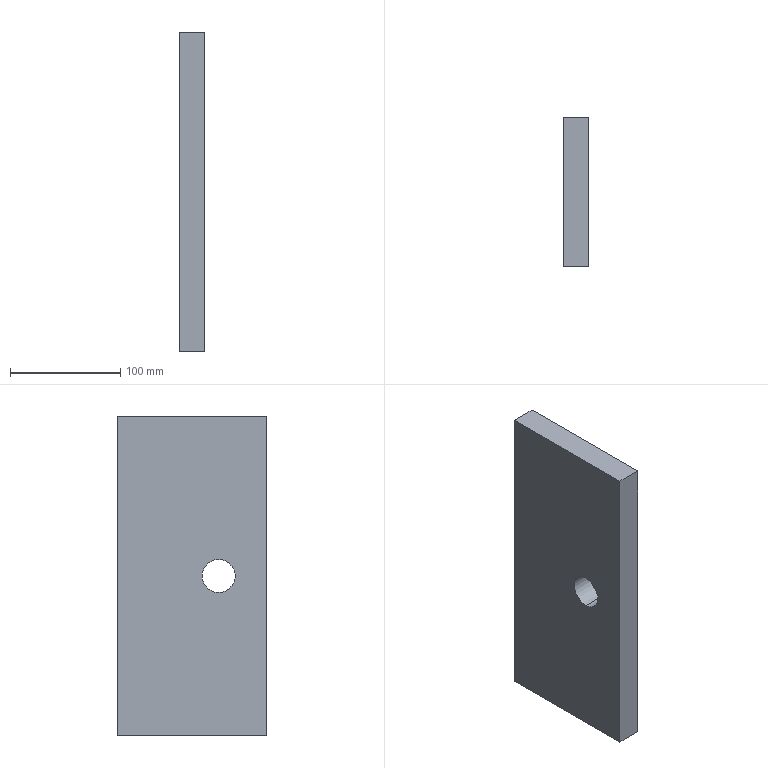Part | SolidWorks | features BaseBody 1 | 1 solid | 13 faces | box 22.77 x 135.5 x 290 mm | volume 870909 mm3 | plane 8 | cylinder 5 | commonest cylinder face diameters 73.25 x3 30 x2
STEP:
#1=CARTESIAN_POINT('',(-12.5,-26.5,-15.));
#2=VERTEX_POINT('',#1);
#3=CARTESIAN_POINT('',(-12.5,-26.5,15.));
#4=VERTEX_POINT('',#3);
#5=CARTESIAN_POINT('',(-12.5,-26.5,0.));
#6=DIRECTION('',(-1.,0.,0.));
#7=DIRECTION('',(0.,0.,-1.));
#8=AXIS2_PLACEMENT_3D('',#5,#6,#7);
#9=CIRCLE('',#8,15.);
#10=EDGE_CURVE('',#2,#4,#9,.T.);
#11=ORIENTED_EDGE('',*,*,#10,.T.);
#12=CARTESIAN_POINT('',(8.04,-26.5,15.));
#13=VERTEX_POINT('',#12);
#14=CARTESIAN_POINT('',(-12.501,-26.5,15.));
#15=DIRECTION('',(1.,0.,0.));
#16=VECTOR('',#15,1000.);
#17=LINE('',#14,#16);
#18=EDGE_CURVE('',#4,#13,#17,.T.);
#19=ORIENTED_EDGE('',*,*,#18,.T.);
#20=CARTESIAN_POINT('',(8.04,-26.5,-15.));
#21=VERTEX_POINT('',#20);
#22=CARTESIAN_POINT('',(8.04,-26.5,0.));
#23=DIRECTION('',(-1.,0.,0.));
#24=DIRECTION('',(0.,0.,-1.));
#25=AXIS2_PLACEMENT_3D('',#22,#23,#24);
#26=CIRCLE('',#25,15.);
#27=EDGE_CURVE('',#21,#13,#26,.T.);
#28=ORIENTED_EDGE('',*,*,#27,.F.);
#29=CARTESIAN_POINT('',(-12.501,-26.5,-15.));
#30=DIRECTION('',(1.,0.,0.));
#31=VECTOR('',#30,1000.);
#32=LINE('',#29,#31);
#33=EDGE_CURVE('',#2,#21,#32,.T.);
#34=ORIENTED_EDGE('',*,*,#33,.F.);
#35=EDGE_LOOP('',(#11,#19,#28,#34));
#36=FACE_OUTER_BOUND('',#35,.T.);
#37=CARTESIAN_POINT('',(-12.501,-26.5,0.));
#38=DIRECTION('',(1.,0.,0.));
#39=DIRECTION('',(0.,0.,-1.));
#40=AXIS2_PLACEMENT_3D('',#37,#38,#39);
#41=CYLINDRICAL_SURFACE('',#40,15.);
#42=ADVANCED_FACE('',(#36),#41,.F.);
#43=CARTESIAN_POINT('',(8.04,-26.5,36.625));
#44=VERTEX_POINT('',#43);
#45=CARTESIAN_POINT('',(8.04,-61.,12.294));
#46=VERTEX_POINT('',#45);
#47=CARTESIAN_POINT('',(8.04,-26.5,0.));
#48=DIRECTION('',(1.,0.,0.));
#49=DIRECTION('',(0.,0.,-1.));
#50=AXIS2_PLACEMENT_3D('',#47,#48,#49);
#51=CIRCLE('',#50,36.625);
#52=EDGE_CURVE('',#44,#46,#51,.T.);
#53=ORIENTED_EDGE('',*,*,#52,.F.);
#54=CARTESIAN_POINT('',(10.27,-26.5,36.625));
#55=VERTEX_POINT('',#54);
#56=CARTESIAN_POINT('',(8.04,-26.5,36.625));
#57=DIRECTION('',(1.,0.,0.));
#58=VECTOR('',#57,1000.);
#59=LINE('',#56,#58);
#60=EDGE_CURVE('',#44,#55,#59,.T.);
#61=ORIENTED_EDGE('',*,*,#60,.T.);
#62=CARTESIAN_POINT('',(10.27,-61.,12.294));
#63=VERTEX_POINT('',#62);
#64=CARTESIAN_POINT('',(10.27,-26.5,0.));
#65=DIRECTION('',(1.,0.,0.));
#66=DIRECTION('',(0.,0.,-1.));
#67=AXIS2_PLACEMENT_3D('',#64,#65,#66);
#68=CIRCLE('',#67,36.625);
#69=EDGE_CURVE('',#55,#63,#68,.T.);
#70=ORIENTED_EDGE('',*,*,#69,.T.);
#71=CARTESIAN_POINT('',(8.04,-61.,12.294));
#72=DIRECTION('',(1.,0.,0.));
#73=VECTOR('',#72,1000.);
#74=LINE('',#71,#73);
#75=EDGE_CURVE('',#46,#63,#74,.T.);
#76=ORIENTED_EDGE('',*,*,#75,.F.);
#77=EDGE_LOOP('',(#53,#61,#70,#76));
#78=FACE_OUTER_BOUND('',#77,.T.);
#79=CARTESIAN_POINT('',(8.04,-26.5,0.));
#80=DIRECTION('',(1.,0.,0.));
#81=DIRECTION('',(0.,0.,-1.));
#82=AXIS2_PLACEMENT_3D('',#79,#80,#81);
#83=CYLINDRICAL_SURFACE('',#82,36.625);
#84=ADVANCED_FACE('',(#78),#83,.F.);
#85=ORIENTED_EDGE('',*,*,#60,.F.);
#86=CARTESIAN_POINT('',(8.04,-26.5,-36.625));
#87=VERTEX_POINT('',#86);
#88=CARTESIAN_POINT('',(8.04,-26.5,0.));
#89=DIRECTION('',(1.,0.,0.));
#90=DIRECTION('',(0.,0.,-1.));
#91=AXIS2_PLACEMENT_3D('',#88,#89,#90);
#92=CIRCLE('',#91,36.625);
#93=EDGE_CURVE('',#87,#44,#92,.T.);
#94=ORIENTED_EDGE('',*,*,#93,.F.);
#95=CARTESIAN_POINT('',(10.27,-26.5,-36.625));
#96=VERTEX_POINT('',#95);
#97=CARTESIAN_POINT('',(8.04,-26.5,-36.625));
#98=DIRECTION('',(1.,0.,0.));
#99=VECTOR('',#98,1000.);
#100=LINE('',#97,#99);
#101=EDGE_CURVE('',#87,#96,#100,.T.);
#102=ORIENTED_EDGE('',*,*,#101,.T.);
#103=CARTESIAN_POINT('',(10.27,-26.5,0.));
#104=DIRECTION('',(1.,0.,0.));
#105=DIRECTION('',(0.,0.,-1.));
#106=AXIS2_PLACEMENT_3D('',#103,#104,#105);
#107=CIRCLE('',#106,36.625);
#108=EDGE_CURVE('',#96,#55,#107,.T.);
#109=ORIENTED_EDGE('',*,*,#108,.T.);
#110=EDGE_LOOP('',(#85,#94,#102,#109));
#111=FACE_OUTER_BOUND('',#110,.T.);
#112=CARTESIAN_POINT('',(8.04,-26.5,0.));
#113=DIRECTION('',(1.,0.,0.));
#114=DIRECTION('',(0.,0.,-1.));
#115=AXIS2_PLACEMENT_3D('',#112,#113,#114);
#116=CYLINDRICAL_SURFACE('',#115,36.625);
#117=ADVANCED_FACE('',(#111),#116,.F.);
#118=ORIENTED_EDGE('',*,*,#27,.T.);
#119=CARTESIAN_POINT('',(8.04,-26.5,0.));
#120=DIRECTION('',(-1.,0.,0.));
#121=DIRECTION('',(0.,0.,-1.));
#122=AXIS2_PLACEMENT_3D('',#119,#120,#121);
#123=CIRCLE('',#122,15.);
#124=EDGE_CURVE('',#13,#21,#123,.T.);
#125=ORIENTED_EDGE('',*,*,#124,.T.);
#126=EDGE_LOOP('',(#118,#125));
#127=FACE_BOUND('',#126,.T.);
#128=CARTESIAN_POINT('',(8.04,-61.,-12.294));
#129=VERTEX_POINT('',#128);
#130=CARTESIAN_POINT('',(8.04,-26.5,0.));
#131=DIRECTION('',(1.,0.,0.));
#132=DIRECTION('',(0.,0.,-1.));
#133=AXIS2_PLACEMENT_3D('',#130,#131,#132);
#134=CIRCLE('',#133,36.625);
#135=EDGE_CURVE('',#129,#87,#134,.T.);
#136=ORIENTED_EDGE('',*,*,#135,.T.);
#137=ORIENTED_EDGE('',*,*,#93,.T.);
#138=ORIENTED_EDGE('',*,*,#52,.T.);
#139=CARTESIAN_POINT('',(8.04,-61.,0.));
#140=DIRECTION('',(0.,0.,-1.));
#141=VECTOR('',#140,1000.);
#142=LINE('',#139,#141);
#143=EDGE_CURVE('',#46,#129,#142,.T.);
#144=ORIENTED_EDGE('',*,*,#143,.T.);
#145=EDGE_LOOP('',(#136,#137,#138,#144));
#146=FACE_OUTER_BOUND('',#145,.T.);
#147=CARTESIAN_POINT('',(8.04,-26.5,0.));
#148=DIRECTION('',(1.,0.,0.));
#149=DIRECTION('',(0.,0.,-1.));
#150=AXIS2_PLACEMENT_3D('',#147,#148,#149);
#151=PLANE('',#150);
#152=ADVANCED_FACE('',(#127,#146),#151,.T.);
#153=ORIENTED_EDGE('',*,*,#101,.F.);
#154=ORIENTED_EDGE('',*,*,#135,.F.);
#155=CARTESIAN_POINT('',(10.27,-61.,-12.294));
#156=VERTEX_POINT('',#155);
#157=CARTESIAN_POINT('',(8.04,-61.,-12.294));
#158=DIRECTION('',(-1.,0.,0.));
#159=VECTOR('',#158,1000.);
#160=LINE('',#157,#159);
#161=EDGE_CURVE('',#156,#129,#160,.T.);
#162=ORIENTED_EDGE('',*,*,#161,.F.);
#163=CARTESIAN_POINT('',(10.27,-26.5,0.));
#164=DIRECTION('',(1.,0.,0.));
#165=DIRECTION('',(0.,0.,-1.));
#166=AXIS2_PLACEMENT_3D('',#163,#164,#165);
#167=CIRCLE('',#166,36.625);
#168=EDGE_CURVE('',#156,#96,#167,.T.);
#169=ORIENTED_EDGE('',*,*,#168,.T.);
#170=EDGE_LOOP('',(#153,#154,#162,#169));
#171=FACE_OUTER_BOUND('',#170,.T.);
#172=CARTESIAN_POINT('',(8.04,-26.5,0.));
#173=DIRECTION('',(1.,0.,0.));
#174=DIRECTION('',(0.,0.,-1.));
#175=AXIS2_PLACEMENT_3D('',#172,#173,#174);
#176=CYLINDRICAL_SURFACE('',#175,36.625);
#177=ADVANCED_FACE('',(#171),#176,.F.);
#178=ORIENTED_EDGE('',*,*,#18,.F.);
#179=CARTESIAN_POINT('',(-12.5,-26.5,0.));
#180=DIRECTION('',(-1.,0.,0.));
#181=DIRECTION('',(0.,0.,-1.));
#182=AXIS2_PLACEMENT_3D('',#179,#180,#181);
#183=CIRCLE('',#182,15.);
#184=EDGE_CURVE('',#4,#2,#183,.T.);
#185=ORIENTED_EDGE('',*,*,#184,.T.);
#186=ORIENTED_EDGE('',*,*,#33,.T.);
#187=ORIENTED_EDGE('',*,*,#124,.F.);
#188=EDGE_LOOP('',(#178,#185,#186,#187));
#189=FACE_OUTER_BOUND('',#188,.T.);
#190=CARTESIAN_POINT('',(-12.501,-26.5,0.));
#191=DIRECTION('',(1.,0.,0.));
#192=DIRECTION('',(0.,0.,-1.));
#193=AXIS2_PLACEMENT_3D('',#190,#191,#192);
#194=CYLINDRICAL_SURFACE('',#193,15.);
#195=ADVANCED_FACE('',(#189),#194,.F.);
#196=CARTESIAN_POINT('',(10.27,65.5,-145.));
#197=VERTEX_POINT('',#196);
#198=CARTESIAN_POINT('',(10.27,65.5,145.));
#199=VERTEX_POINT('',#198);
#200=CARTESIAN_POINT('',(10.27,65.5,-145.));
#201=DIRECTION('',(0.,0.,1.));
#202=VECTOR('',#201,1000.);
#203=LINE('',#200,#202);
#204=EDGE_CURVE('',#197,#199,#203,.T.);
#205=ORIENTED_EDGE('',*,*,#204,.F.);
#206=CARTESIAN_POINT('',(-12.5,65.5,-145.));
#207=VERTEX_POINT('',#206);
#208=CARTESIAN_POINT('',(-12.5,65.5,-145.));
#209=DIRECTION('',(-1.,0.,0.));
#210=VECTOR('',#209,1000.);
#211=LINE('',#208,#210);
#212=EDGE_CURVE('',#197,#207,#211,.T.);
#213=ORIENTED_EDGE('',*,*,#212,.T.);
#214=CARTESIAN_POINT('',(-12.5,65.5,145.));
#215=VERTEX_POINT('',#214);
#216=CARTESIAN_POINT('',(-12.5,65.5,145.));
#217=DIRECTION('',(0.,0.,-1.));
#218=VECTOR('',#217,1000.);
#219=LINE('',#216,#218);
#220=EDGE_CURVE('',#215,#207,#219,.T.);
#221=ORIENTED_EDGE('',*,*,#220,.F.);
#222=CARTESIAN_POINT('',(-12.5,65.5,145.));
#223=DIRECTION('',(-1.,0.,0.));
#224=VECTOR('',#223,1000.);
#225=LINE('',#222,#224);
#226=EDGE_CURVE('',#199,#215,#225,.T.);
#227=ORIENTED_EDGE('',*,*,#226,.F.);
#228=EDGE_LOOP('',(#205,#213,#221,#227));
#229=FACE_OUTER_BOUND('',#228,.T.);
#230=CARTESIAN_POINT('',(-12.5,65.5,145.));
#231=DIRECTION('',(0.,-1.,0.));
#232=DIRECTION('',(0.,0.,-1.));
#233=AXIS2_PLACEMENT_3D('',#230,#231,#232);
#234=PLANE('',#233);
#235=ADVANCED_FACE('',(#229),#234,.F.);
#236=CARTESIAN_POINT('',(10.27,-70.,145.));
#237=VERTEX_POINT('',#236);
#238=CARTESIAN_POINT('',(-12.5,-70.,145.));
#239=VERTEX_POINT('',#238);
#240=CARTESIAN_POINT('',(10.27,-70.,145.));
#241=DIRECTION('',(-1.,0.,0.));
#242=VECTOR('',#241,1000.);
#243=LINE('',#240,#242);
#244=EDGE_CURVE('',#237,#239,#243,.T.);
#245=ORIENTED_EDGE('',*,*,#244,.F.);
#246=CARTESIAN_POINT('',(10.27,65.5,145.));
#247=DIRECTION('',(0.,-1.,0.));
#248=VECTOR('',#247,1000.);
#249=LINE('',#246,#248);
#250=EDGE_CURVE('',#199,#237,#249,.T.);
#251=ORIENTED_EDGE('',*,*,#250,.F.);
#252=ORIENTED_EDGE('',*,*,#226,.T.);
#253=CARTESIAN_POINT('',(-12.5,-65.5,145.));
#254=DIRECTION('',(0.,-1.,0.));
#255=VECTOR('',#254,1000.);
#256=LINE('',#253,#255);
#257=EDGE_CURVE('',#215,#239,#256,.T.);
#258=ORIENTED_EDGE('',*,*,#257,.T.);
#259=EDGE_LOOP('',(#245,#251,#252,#258));
#260=FACE_OUTER_BOUND('',#259,.T.);
#261=CARTESIAN_POINT('',(0.,0.,145.));
#262=DIRECTION('',(0.,0.,-1.));
#263=DIRECTION('',(-1.,0.,0.));
#264=AXIS2_PLACEMENT_3D('',#261,#262,#263);
#265=PLANE('',#264);
#266=ADVANCED_FACE('',(#260),#265,.F.);
#267=CARTESIAN_POINT('',(-12.5,-70.,-145.));
#268=VERTEX_POINT('',#267);
#269=CARTESIAN_POINT('',(10.27,-70.,-145.));
#270=VERTEX_POINT('',#269);
#271=CARTESIAN_POINT('',(-12.5,-70.,-145.));
#272=DIRECTION('',(1.,0.,0.));
#273=VECTOR('',#272,1000.);
#274=LINE('',#271,#273);
#275=EDGE_CURVE('',#268,#270,#274,.T.);
#276=ORIENTED_EDGE('',*,*,#275,.F.);
#277=CARTESIAN_POINT('',(-12.5,-65.5,-145.));
#278=DIRECTION('',(0.,-1.,0.));
#279=VECTOR('',#278,1000.);
#280=LINE('',#277,#279);
#281=EDGE_CURVE('',#207,#268,#280,.T.);
#282=ORIENTED_EDGE('',*,*,#281,.F.);
#283=ORIENTED_EDGE('',*,*,#212,.F.);
#284=CARTESIAN_POINT('',(10.27,-65.5,-145.));
#285=DIRECTION('',(0.,1.,0.));
#286=VECTOR('',#285,1000.);
#287=LINE('',#284,#286);
#288=EDGE_CURVE('',#270,#197,#287,.T.);
#289=ORIENTED_EDGE('',*,*,#288,.F.);
#290=EDGE_LOOP('',(#276,#282,#283,#289));
#291=FACE_OUTER_BOUND('',#290,.T.);
#292=CARTESIAN_POINT('',(0.,0.,-145.));
#293=DIRECTION('',(0.,0.,-1.));
#294=DIRECTION('',(-1.,0.,0.));
#295=AXIS2_PLACEMENT_3D('',#292,#293,#294);
#296=PLANE('',#295);
#297=ADVANCED_FACE('',(#291),#296,.T.);
#298=CARTESIAN_POINT('',(-12.5,-70.,145.));
#299=DIRECTION('',(0.,0.,-1.));
#300=VECTOR('',#299,1000.);
#301=LINE('',#298,#300);
#302=EDGE_CURVE('',#239,#268,#301,.T.);
#303=ORIENTED_EDGE('',*,*,#302,.F.);
#304=ORIENTED_EDGE('',*,*,#257,.F.);
#305=ORIENTED_EDGE('',*,*,#220,.T.);
#306=ORIENTED_EDGE('',*,*,#281,.T.);
#307=EDGE_LOOP('',(#303,#304,#305,#306));
#308=FACE_OUTER_BOUND('',#307,.T.);
#309=ORIENTED_EDGE('',*,*,#10,.F.);
#310=ORIENTED_EDGE('',*,*,#184,.F.);
#311=EDGE_LOOP('',(#309,#310));
#312=FACE_BOUND('',#311,.T.);
#313=CARTESIAN_POINT('',(-12.5,-65.5,145.));
#314=DIRECTION('',(1.,0.,0.));
#315=DIRECTION('',(0.,0.,-1.));
#316=AXIS2_PLACEMENT_3D('',#313,#314,#315);
#317=PLANE('',#316);
#318=ADVANCED_FACE('',(#308,#312),#317,.F.);
#319=CARTESIAN_POINT('',(10.27,-61.,-145.));
#320=DIRECTION('',(0.,0.,1.));
#321=VECTOR('',#320,1000.);
#322=LINE('',#319,#321);
#323=EDGE_CURVE('',#156,#63,#322,.T.);
#324=ORIENTED_EDGE('',*,*,#323,.T.);
#325=ORIENTED_EDGE('',*,*,#69,.F.);
#326=ORIENTED_EDGE('',*,*,#108,.F.);
#327=ORIENTED_EDGE('',*,*,#168,.F.);
#328=EDGE_LOOP('',(#324,#325,#326,#327));
#329=FACE_BOUND('',#328,.T.);
#330=ORIENTED_EDGE('',*,*,#250,.T.);
#331=CARTESIAN_POINT('',(10.27,-70.,-145.));
#332=DIRECTION('',(0.,0.,1.));
#333=VECTOR('',#332,1000.);
#334=LINE('',#331,#333);
#335=EDGE_CURVE('',#270,#237,#334,.T.);
#336=ORIENTED_EDGE('',*,*,#335,.F.);
#337=ORIENTED_EDGE('',*,*,#288,.T.);
#338=ORIENTED_EDGE('',*,*,#204,.T.);
#339=EDGE_LOOP('',(#330,#336,#337,#338));
#340=FACE_OUTER_BOUND('',#339,.T.);
#341=CARTESIAN_POINT('',(10.27,0.,0.));
#342=DIRECTION('',(1.,0.,0.));
#343=DIRECTION('',(0.,0.,-1.));
#344=AXIS2_PLACEMENT_3D('',#341,#342,#343);
#345=PLANE('',#344);
#346=ADVANCED_FACE('',(#329,#340),#345,.T.);
#347=ORIENTED_EDGE('',*,*,#323,.F.);
#348=ORIENTED_EDGE('',*,*,#161,.T.);
#349=ORIENTED_EDGE('',*,*,#143,.F.);
#350=ORIENTED_EDGE('',*,*,#75,.T.);
#351=EDGE_LOOP('',(#347,#348,#349,#350));
#352=FACE_OUTER_BOUND('',#351,.T.);
#353=CARTESIAN_POINT('',(0.,-61.,0.));
#354=DIRECTION('',(0.,-1.,0.));
#355=DIRECTION('',(0.,0.,-1.));
#356=AXIS2_PLACEMENT_3D('',#353,#354,#355);
#357=PLANE('',#356);
#358=ADVANCED_FACE('',(#352),#357,.F.);
#359=ORIENTED_EDGE('',*,*,#275,.T.);
#360=ORIENTED_EDGE('',*,*,#335,.T.);
#361=ORIENTED_EDGE('',*,*,#244,.T.);
#362=ORIENTED_EDGE('',*,*,#302,.T.);
#363=EDGE_LOOP('',(#359,#360,#361,#362));
#364=FACE_OUTER_BOUND('',#363,.T.);
#365=CARTESIAN_POINT('',(0.,-70.,0.));
#366=DIRECTION('',(0.,-1.,0.));
#367=DIRECTION('',(0.,0.,-1.));
#368=AXIS2_PLACEMENT_3D('',#365,#366,#367);
#369=PLANE('',#368);
#370=ADVANCED_FACE('',(#364),#369,.T.);
#371=CLOSED_SHELL('',(#42,#84,#117,#152,#177,#195,#235,#266,#297,#318,#346,#358,#370));
#372=MANIFOLD_SOLID_BREP('',#371);
#373=CARTESIAN_POINT('',(0.,0.,0.));
#374=DIRECTION('',(0.,0.,1.));
#375=DIRECTION('',(1.,0.,0.));
#376=AXIS2_PLACEMENT_3D('',#373,#374,#375);
#377=(LENGTH_UNIT()NAMED_UNIT(*)SI_UNIT(.MILLI.,.METRE.));
#378=UNCERTAINTY_MEASURE_WITH_UNIT(LENGTH_MEASURE(0.00001),#377,'','');
#379=(NAMED_UNIT(*)PLANE_ANGLE_UNIT()SI_UNIT($,.RADIAN.));
#380=(NAMED_UNIT(*)SI_UNIT($,.STERADIAN.)SOLID_ANGLE_UNIT());
#381=(GEOMETRIC_REPRESENTATION_CONTEXT(3)GLOBAL_UNCERTAINTY_ASSIGNED_CONTEXT((#378))GLOBAL_UNIT_ASSIGNED_CONTEXT((#377,#379,#380))REPRESENTATION_CONTEXT('',''));
#382=ADVANCED_BREP_SHAPE_REPRESENTATION('',(#372,#376),#381);